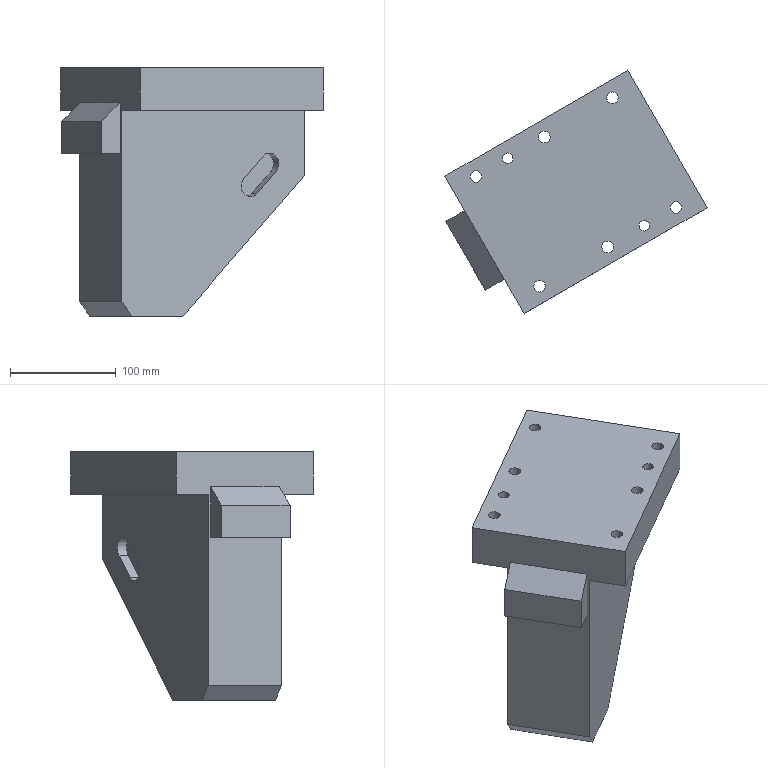Part | NX | features solid 2 | 1 solid | 47 faces | box 248.205 x 229.904 x 235 mm | volume 3610096 mm3 | plane 29 | cylinder 18 | commonest cylinder face diameters 11 x6 17 x6 20 x4 10 x2
STEP:
#1=CARTESIAN_POINT('',(-1183.369,-2.122,138.943));
#2=VERTEX_POINT('',#1);
#3=CARTESIAN_POINT('',(-1165.421,8.24,138.943));
#4=VERTEX_POINT('',#3);
#5=CARTESIAN_POINT('',(-1169.752,5.74,138.943));
#6=DIRECTION('',(-0.866,-0.5,0.));
#7=VECTOR('',#6,1000.);
#8=LINE('',#5,#7);
#9=EDGE_CURVE('',#2,#4,#8,.F.);
#10=ORIENTED_EDGE('',*,*,#9,.T.);
#11=CARTESIAN_POINT('',(-1127.921,-56.712,138.943));
#12=VERTEX_POINT('',#11);
#13=CARTESIAN_POINT('',(-1088.171,-125.561,138.943));
#14=DIRECTION('',(-0.5,0.866,0.));
#15=VECTOR('',#14,1000.);
#16=LINE('',#13,#15);
#17=EDGE_CURVE('',#12,#4,#16,.T.);
#18=ORIENTED_EDGE('',*,*,#17,.F.);
#19=CARTESIAN_POINT('',(-1145.869,-67.074,138.943));
#20=VERTEX_POINT('',#19);
#21=CARTESIAN_POINT('',(-1132.252,-59.212,138.943));
#22=DIRECTION('',(0.866,0.5,0.));
#23=VECTOR('',#22,1000.);
#24=LINE('',#21,#23);
#25=EDGE_CURVE('',#20,#12,#24,.T.);
#26=ORIENTED_EDGE('',*,*,#25,.F.);
#27=CARTESIAN_POINT('',(-1145.869,-67.074,138.943));
#28=DIRECTION('',(-0.5,0.866,0.));
#29=VECTOR('',#28,1000.);
#30=LINE('',#27,#29);
#31=EDGE_CURVE('',#20,#2,#30,.T.);
#32=ORIENTED_EDGE('',*,*,#31,.T.);
#33=EDGE_LOOP('',(#10,#18,#26,#32));
#34=FACE_BOUND('',#33,.T.);
#35=CARTESIAN_POINT('',(-1088.171,-125.561,138.943));
#36=DIRECTION('',(0.,0.,1.));
#37=DIRECTION('',(0.5,-0.866,0.));
#38=AXIS2_PLACEMENT_3D('',#35,#36,#37);
#39=PLANE('',#38);
#40=ADVANCED_FACE('',(#34),#39,.F.);
#41=CARTESIAN_POINT('',(-1145.869,-67.074,169.58));
#42=VERTEX_POINT('',#41);
#43=CARTESIAN_POINT('',(-1127.921,-56.712,186.97));
#44=VERTEX_POINT('',#43);
#45=CARTESIAN_POINT('',(-1129.327,-57.524,185.608));
#46=DIRECTION('',(0.6634,0.383,0.6428));
#47=VECTOR('',#46,1000.);
#48=LINE('',#45,#47);
#49=EDGE_CURVE('',#42,#44,#48,.T.);
#50=ORIENTED_EDGE('',*,*,#49,.T.);
#51=CARTESIAN_POINT('',(-1165.421,8.24,186.97));
#52=VERTEX_POINT('',#51);
#53=CARTESIAN_POINT('',(-1126.671,-58.877,186.97));
#54=DIRECTION('',(0.5,-0.866,0.));
#55=VECTOR('',#54,1000.);
#56=LINE('',#53,#55);
#57=EDGE_CURVE('',#52,#44,#56,.T.);
#58=ORIENTED_EDGE('',*,*,#57,.F.);
#59=CARTESIAN_POINT('',(-1183.369,-2.122,169.58));
#60=VERTEX_POINT('',#59);
#61=CARTESIAN_POINT('',(-1166.827,7.428,185.608));
#62=DIRECTION('',(-0.6634,-0.383,-0.6428));
#63=VECTOR('',#62,1000.);
#64=LINE('',#61,#63);
#65=EDGE_CURVE('',#60,#52,#64,.F.);
#66=ORIENTED_EDGE('',*,*,#65,.F.);
#67=CARTESIAN_POINT('',(-1145.869,-67.074,169.58));
#68=DIRECTION('',(0.5,-0.866,0.));
#69=VECTOR('',#68,1000.);
#70=LINE('',#67,#69);
#71=EDGE_CURVE('',#42,#60,#70,.F.);
#72=ORIENTED_EDGE('',*,*,#71,.F.);
#73=EDGE_LOOP('',(#50,#58,#66,#72));
#74=FACE_BOUND('',#73,.T.);
#75=CARTESIAN_POINT('',(-1128.077,-59.689,185.608));
#76=DIRECTION('',(0.5567,0.3214,-0.766));
#77=DIRECTION('',(-0.6313,-0.4358,-0.6416));
#78=AXIS2_PLACEMENT_3D('',#75,#76,#77);
#79=PLANE('',#78);
#80=ADVANCED_FACE('',(#74),#79,.F.);
#81=CARTESIAN_POINT('',(-998.759,14.973,101.136));
#82=VERTEX_POINT('',#81);
#83=CARTESIAN_POINT('',(-1011.006,7.902,115.279));
#84=VERTEX_POINT('',#83);
#85=CARTESIAN_POINT('',(-1004.882,11.438,108.208));
#86=DIRECTION('',(0.5,-0.866,0.));
#87=DIRECTION('',(0.866,0.5,0.));
#88=AXIS2_PLACEMENT_3D('',#85,#86,#87);
#89=CIRCLE('',#88,10.);
#90=EDGE_CURVE('',#82,#84,#89,.F.);
#91=ORIENTED_EDGE('',*,*,#90,.T.);
#92=CARTESIAN_POINT('',(-992.635,18.509,136.492));
#93=VERTEX_POINT('',#92);
#94=CARTESIAN_POINT('',(-1017.13,4.367,108.208));
#95=DIRECTION('',(0.6124,0.3536,0.7071));
#96=VECTOR('',#95,1000.);
#97=LINE('',#94,#96);
#98=EDGE_CURVE('',#93,#84,#97,.F.);
#99=ORIENTED_EDGE('',*,*,#98,.F.);
#100=CARTESIAN_POINT('',(-980.387,25.58,122.35));
#101=VERTEX_POINT('',#100);
#102=CARTESIAN_POINT('',(-986.511,22.044,129.421));
#103=DIRECTION('',(0.5,-0.866,0.));
#104=DIRECTION('',(0.866,0.5,0.));
#105=AXIS2_PLACEMENT_3D('',#102,#103,#104);
#106=CIRCLE('',#105,10.);
#107=EDGE_CURVE('',#93,#101,#106,.F.);
#108=ORIENTED_EDGE('',*,*,#107,.T.);
#109=CARTESIAN_POINT('',(-924.354,57.931,187.052));
#110=DIRECTION('',(-0.6124,-0.3536,-0.7071));
#111=VECTOR('',#110,1000.);
#112=LINE('',#109,#111);
#113=EDGE_CURVE('',#82,#101,#112,.F.);
#114=ORIENTED_EDGE('',*,*,#113,.F.);
#115=EDGE_LOOP('',(#91,#99,#108,#114));
#116=FACE_BOUND('',#115,.T.);
#117=CARTESIAN_POINT('',(-1126.671,-58.877,-1.401));
#118=VERTEX_POINT('',#117);
#119=CARTESIAN_POINT('',(-1116.79,-53.172,-15.));
#120=VERTEX_POINT('',#119);
#121=CARTESIAN_POINT('',(-1116.129,-52.791,-15.909));
#122=DIRECTION('',(-0.5567,-0.3214,0.766));
#123=VECTOR('',#122,1000.);
#124=LINE('',#121,#123);
#125=EDGE_CURVE('',#118,#120,#124,.F.);
#126=ORIENTED_EDGE('',*,*,#125,.T.);
#127=CARTESIAN_POINT('',(-1068.717,-25.417,-15.));
#128=VERTEX_POINT('',#127);
#129=CARTESIAN_POINT('',(-746.06,160.869,-15.));
#130=DIRECTION('',(-0.866,-0.5,0.));
#131=VECTOR('',#130,1000.);
#132=LINE('',#129,#131);
#133=EDGE_CURVE('',#120,#128,#132,.F.);
#134=ORIENTED_EDGE('',*,*,#133,.T.);
#135=CARTESIAN_POINT('',(-953.466,41.123,118.08));
#136=VERTEX_POINT('',#135);
#137=CARTESIAN_POINT('',(-1050.063,-14.647,6.54));
#138=DIRECTION('',(-0.6124,-0.3536,-0.7071));
#139=VECTOR('',#138,1000.);
#140=LINE('',#137,#139);
#141=EDGE_CURVE('',#128,#136,#140,.F.);
#142=ORIENTED_EDGE('',*,*,#141,.T.);
#143=CARTESIAN_POINT('',(-953.466,41.123,180.));
#144=VERTEX_POINT('',#143);
#145=CARTESIAN_POINT('',(-953.466,41.123,-270.576));
#146=DIRECTION('',(0.,0.,-1.));
#147=VECTOR('',#146,1000.);
#148=LINE('',#145,#147);
#149=EDGE_CURVE('',#136,#144,#148,.F.);
#150=ORIENTED_EDGE('',*,*,#149,.T.);
#151=CARTESIAN_POINT('',(-1126.671,-58.877,180.));
#152=VERTEX_POINT('',#151);
#153=CARTESIAN_POINT('',(-746.06,160.869,180.));
#154=DIRECTION('',(0.866,0.5,0.));
#155=VECTOR('',#154,1000.);
#156=LINE('',#153,#155);
#157=EDGE_CURVE('',#144,#152,#156,.F.);
#158=ORIENTED_EDGE('',*,*,#157,.T.);
#159=CARTESIAN_POINT('',(-1126.671,-58.877,-5.827));
#160=DIRECTION('',(0.,0.,-1.));
#161=VECTOR('',#160,1000.);
#162=LINE('',#159,#161);
#163=EDGE_CURVE('',#118,#152,#162,.F.);
#164=ORIENTED_EDGE('',*,*,#163,.F.);
#165=EDGE_LOOP('',(#126,#134,#142,#150,#158,#164));
#166=FACE_BOUND('',#165,.T.);
#167=CARTESIAN_POINT('',(-746.06,160.869,-18.824));
#168=DIRECTION('',(0.5,-0.866,0.));
#169=DIRECTION('',(0.8627,0.4981,-0.08716));
#170=AXIS2_PLACEMENT_3D('',#167,#168,#169);
#171=PLANE('',#170);
#172=ADVANCED_FACE('',(#116,#166),#171,.T.);
#173=CARTESIAN_POINT('',(-1016.006,16.562,115.279));
#174=VERTEX_POINT('',#173);
#175=CARTESIAN_POINT('',(-1003.759,23.634,101.136));
#176=VERTEX_POINT('',#175);
#177=CARTESIAN_POINT('',(-1009.882,20.098,108.208));
#178=DIRECTION('',(0.5,-0.866,0.));
#179=DIRECTION('',(0.866,0.5,0.));
#180=AXIS2_PLACEMENT_3D('',#177,#178,#179);
#181=CIRCLE('',#180,10.);
#182=EDGE_CURVE('',#174,#176,#181,.T.);
#183=ORIENTED_EDGE('',*,*,#182,.T.);
#184=CARTESIAN_POINT('',(-985.387,34.24,122.35));
#185=VERTEX_POINT('',#184);
#186=CARTESIAN_POINT('',(-1052.748,-4.651,44.568));
#187=DIRECTION('',(-0.6124,-0.3536,-0.7071));
#188=VECTOR('',#187,1000.);
#189=LINE('',#186,#188);
#190=EDGE_CURVE('',#176,#185,#189,.F.);
#191=ORIENTED_EDGE('',*,*,#190,.T.);
#192=CARTESIAN_POINT('',(-997.635,27.169,136.492));
#193=VERTEX_POINT('',#192);
#194=CARTESIAN_POINT('',(-991.511,30.705,129.421));
#195=DIRECTION('',(0.5,-0.866,0.));
#196=DIRECTION('',(0.866,0.5,0.));
#197=AXIS2_PLACEMENT_3D('',#194,#195,#196);
#198=CIRCLE('',#197,10.);
#199=EDGE_CURVE('',#185,#193,#198,.T.);
#200=ORIENTED_EDGE('',*,*,#199,.T.);
#201=CARTESIAN_POINT('',(-1064.996,-11.722,58.71));
#202=DIRECTION('',(-0.6124,-0.3536,-0.7071));
#203=VECTOR('',#202,1000.);
#204=LINE('',#201,#203);
#205=EDGE_CURVE('',#174,#193,#204,.F.);
#206=ORIENTED_EDGE('',*,*,#205,.F.);
#207=EDGE_LOOP('',(#183,#191,#200,#206));
#208=FACE_BOUND('',#207,.T.);
#209=CARTESIAN_POINT('',(-1052.748,-4.651,44.568));
#210=DIRECTION('',(0.5,-0.866,0.));
#211=DIRECTION('',(0.6124,0.3536,0.7071));
#212=AXIS2_PLACEMENT_3D('',#209,#210,#211);
#213=PLANE('',#212);
#214=ADVANCED_FACE('',(#208),#213,.T.);
#215=CARTESIAN_POINT('',(-1046.006,68.524,115.279));
#216=VERTEX_POINT('',#215);
#217=CARTESIAN_POINT('',(-1033.759,75.595,101.136));
#218=VERTEX_POINT('',#217);
#219=CARTESIAN_POINT('',(-1039.882,72.059,108.208));
#220=DIRECTION('',(-0.5,0.866,0.));
#221=DIRECTION('',(-0.8627,-0.4981,0.08716));
#222=AXIS2_PLACEMENT_3D('',#219,#220,#221);
#223=CIRCLE('',#222,10.);
#224=EDGE_CURVE('',#216,#218,#223,.F.);
#225=ORIENTED_EDGE('',*,*,#224,.F.);
#226=CARTESIAN_POINT('',(-1027.635,79.131,136.492));
#227=VERTEX_POINT('',#226);
#228=CARTESIAN_POINT('',(-1052.13,64.988,108.208));
#229=DIRECTION('',(-0.6124,-0.3536,-0.7071));
#230=VECTOR('',#229,1000.);
#231=LINE('',#228,#230);
#232=EDGE_CURVE('',#216,#227,#231,.F.);
#233=ORIENTED_EDGE('',*,*,#232,.T.);
#234=CARTESIAN_POINT('',(-1015.387,86.202,122.35));
#235=VERTEX_POINT('',#234);
#236=CARTESIAN_POINT('',(-1021.511,82.666,129.421));
#237=DIRECTION('',(-0.5,0.866,0.));
#238=DIRECTION('',(-0.8627,-0.4981,0.08716));
#239=AXIS2_PLACEMENT_3D('',#236,#237,#238);
#240=CIRCLE('',#239,10.);
#241=EDGE_CURVE('',#235,#227,#240,.F.);
#242=ORIENTED_EDGE('',*,*,#241,.F.);
#243=CARTESIAN_POINT('',(-1039.882,72.059,94.065));
#244=DIRECTION('',(-0.6124,-0.3536,-0.7071));
#245=VECTOR('',#244,1000.);
#246=LINE('',#243,#245);
#247=EDGE_CURVE('',#218,#235,#246,.F.);
#248=ORIENTED_EDGE('',*,*,#247,.F.);
#249=EDGE_LOOP('',(#225,#233,#242,#248));
#250=FACE_BOUND('',#249,.T.);
#251=CARTESIAN_POINT('',(-1082.748,47.311,44.568));
#252=DIRECTION('',(-0.5,0.866,0.));
#253=DIRECTION('',(0.6124,0.3536,0.7071));
#254=AXIS2_PLACEMENT_3D('',#251,#252,#253);
#255=PLANE('',#254);
#256=ADVANCED_FACE('',(#250),#255,.T.);
#257=ORIENTED_EDGE('',*,*,#113,.T.);
#258=CARTESIAN_POINT('',(-935.387,-52.362,122.35));
#259=DIRECTION('',(-0.5,0.866,0.));
#260=VECTOR('',#259,1000.);
#261=LINE('',#258,#260);
#262=EDGE_CURVE('',#101,#185,#261,.T.);
#263=ORIENTED_EDGE('',*,*,#262,.T.);
#264=ORIENTED_EDGE('',*,*,#190,.F.);
#265=CARTESIAN_POINT('',(-953.759,-62.969,101.136));
#266=DIRECTION('',(-0.5,0.866,0.));
#267=VECTOR('',#266,1000.);
#268=LINE('',#265,#267);
#269=EDGE_CURVE('',#82,#176,#268,.T.);
#270=ORIENTED_EDGE('',*,*,#269,.F.);
#271=EDGE_LOOP('',(#257,#263,#264,#270));
#272=FACE_BOUND('',#271,.T.);
#273=CARTESIAN_POINT('',(-959.882,-66.505,94.065));
#274=DIRECTION('',(-0.6124,-0.3536,0.7071));
#275=DIRECTION('',(-0.4824,-0.5415,-0.6885));
#276=AXIS2_PLACEMENT_3D('',#273,#274,#275);
#277=PLANE('',#276);
#278=ADVANCED_FACE('',(#272),#277,.T.);
#279=ORIENTED_EDGE('',*,*,#107,.F.);
#280=CARTESIAN_POINT('',(-947.635,-59.434,136.492));
#281=DIRECTION('',(-0.5,0.866,0.));
#282=VECTOR('',#281,1000.);
#283=LINE('',#280,#282);
#284=EDGE_CURVE('',#93,#193,#283,.T.);
#285=ORIENTED_EDGE('',*,*,#284,.T.);
#286=ORIENTED_EDGE('',*,*,#199,.F.);
#287=ORIENTED_EDGE('',*,*,#262,.F.);
#288=EDGE_LOOP('',(#279,#285,#286,#287));
#289=FACE_BOUND('',#288,.T.);
#290=CARTESIAN_POINT('',(-941.511,-55.898,129.421));
#291=DIRECTION('',(-0.5,0.866,0.));
#292=DIRECTION('',(-0.8627,-0.4981,0.08716));
#293=AXIS2_PLACEMENT_3D('',#290,#291,#292);
#294=CYLINDRICAL_SURFACE('',#293,10.);
#295=ADVANCED_FACE('',(#289),#294,.F.);
#296=ORIENTED_EDGE('',*,*,#284,.F.);
#297=ORIENTED_EDGE('',*,*,#98,.T.);
#298=CARTESIAN_POINT('',(-966.006,-70.04,115.279));
#299=DIRECTION('',(-0.5,0.866,0.));
#300=VECTOR('',#299,1000.);
#301=LINE('',#298,#300);
#302=EDGE_CURVE('',#84,#174,#301,.T.);
#303=ORIENTED_EDGE('',*,*,#302,.T.);
#304=ORIENTED_EDGE('',*,*,#205,.T.);
#305=EDGE_LOOP('',(#296,#297,#303,#304));
#306=FACE_BOUND('',#305,.T.);
#307=CARTESIAN_POINT('',(-972.13,-73.576,108.208));
#308=DIRECTION('',(-0.6124,-0.3536,0.7071));
#309=DIRECTION('',(-0.4824,-0.5415,-0.6885));
#310=AXIS2_PLACEMENT_3D('',#307,#308,#309);
#311=PLANE('',#310);
#312=ADVANCED_FACE('',(#306),#311,.F.);
#313=ORIENTED_EDGE('',*,*,#302,.F.);
#314=ORIENTED_EDGE('',*,*,#90,.F.);
#315=ORIENTED_EDGE('',*,*,#269,.T.);
#316=ORIENTED_EDGE('',*,*,#182,.F.);
#317=EDGE_LOOP('',(#313,#314,#315,#316));
#318=FACE_BOUND('',#317,.T.);
#319=CARTESIAN_POINT('',(-959.882,-66.505,108.208));
#320=DIRECTION('',(-0.5,0.866,0.));
#321=DIRECTION('',(-0.8627,-0.4981,0.08716));
#322=AXIS2_PLACEMENT_3D('',#319,#320,#321);
#323=CYLINDRICAL_SURFACE('',#322,10.);
#324=ADVANCED_FACE('',(#318),#323,.F.);
#325=ORIENTED_EDGE('',*,*,#241,.T.);
#326=CARTESIAN_POINT('',(-1032.635,87.791,136.492));
#327=VERTEX_POINT('',#326);
#328=CARTESIAN_POINT('',(-1032.635,87.791,136.492));
#329=DIRECTION('',(0.5,-0.866,0.));
#330=VECTOR('',#329,1000.);
#331=LINE('',#328,#330);
#332=EDGE_CURVE('',#227,#327,#331,.F.);
#333=ORIENTED_EDGE('',*,*,#332,.T.);
#334=CARTESIAN_POINT('',(-1020.387,94.862,122.35));
#335=VERTEX_POINT('',#334);
#336=CARTESIAN_POINT('',(-1026.511,91.326,129.421));
#337=DIRECTION('',(-0.5,0.866,0.));
#338=DIRECTION('',(-0.8627,-0.4981,0.08716));
#339=AXIS2_PLACEMENT_3D('',#336,#337,#338);
#340=CIRCLE('',#339,10.);
#341=EDGE_CURVE('',#327,#335,#340,.T.);
#342=ORIENTED_EDGE('',*,*,#341,.T.);
#343=CARTESIAN_POINT('',(-1017.887,90.532,122.35));
#344=DIRECTION('',(0.5,-0.866,0.));
#345=VECTOR('',#344,1000.);
#346=LINE('',#343,#345);
#347=EDGE_CURVE('',#335,#235,#346,.T.);
#348=ORIENTED_EDGE('',*,*,#347,.T.);
#349=EDGE_LOOP('',(#325,#333,#342,#348));
#350=FACE_BOUND('',#349,.T.);
#351=CARTESIAN_POINT('',(-1024.011,86.996,129.421));
#352=DIRECTION('',(-0.5,0.866,0.));
#353=DIRECTION('',(0.8627,0.4981,-0.08716));
#354=AXIS2_PLACEMENT_3D('',#351,#352,#353);
#355=CYLINDRICAL_SURFACE('',#354,10.);
#356=ADVANCED_FACE('',(#350),#355,.F.);
#357=ORIENTED_EDGE('',*,*,#247,.T.);
#358=ORIENTED_EDGE('',*,*,#347,.F.);
#359=CARTESIAN_POINT('',(-1038.759,84.255,101.136));
#360=VERTEX_POINT('',#359);
#361=CARTESIAN_POINT('',(-1044.882,80.72,94.065));
#362=DIRECTION('',(0.6124,0.3536,0.7071));
#363=VECTOR('',#362,1000.);
#364=LINE('',#361,#363);
#365=EDGE_CURVE('',#360,#335,#364,.T.);
#366=ORIENTED_EDGE('',*,*,#365,.F.);
#367=CARTESIAN_POINT('',(-1036.259,79.925,101.136));
#368=DIRECTION('',(-0.5,0.866,0.));
#369=VECTOR('',#368,1000.);
#370=LINE('',#367,#369);
#371=EDGE_CURVE('',#218,#360,#370,.T.);
#372=ORIENTED_EDGE('',*,*,#371,.F.);
#373=EDGE_LOOP('',(#357,#358,#366,#372));
#374=FACE_BOUND('',#373,.T.);
#375=CARTESIAN_POINT('',(-1042.382,76.39,94.065));
#376=DIRECTION('',(-0.6124,-0.3536,0.7071));
#377=DIRECTION('',(0.6124,0.3536,0.7071));
#378=AXIS2_PLACEMENT_3D('',#375,#376,#377);
#379=PLANE('',#378);
#380=ADVANCED_FACE('',(#374),#379,.T.);
#381=CARTESIAN_POINT('',(-1051.006,77.184,115.279));
#382=VERTEX_POINT('',#381);
#383=CARTESIAN_POINT('',(-1044.882,80.72,108.208));
#384=DIRECTION('',(-0.5,0.866,0.));
#385=DIRECTION('',(-0.8627,-0.4981,0.08716));
#386=AXIS2_PLACEMENT_3D('',#383,#384,#385);
#387=CIRCLE('',#386,10.);
#388=EDGE_CURVE('',#360,#382,#387,.T.);
#389=ORIENTED_EDGE('',*,*,#388,.T.);
#390=CARTESIAN_POINT('',(-1041.006,59.864,115.279));
#391=DIRECTION('',(-0.5,0.866,0.));
#392=VECTOR('',#391,1000.);
#393=LINE('',#390,#392);
#394=EDGE_CURVE('',#382,#216,#393,.F.);
#395=ORIENTED_EDGE('',*,*,#394,.T.);
#396=ORIENTED_EDGE('',*,*,#224,.T.);
#397=ORIENTED_EDGE('',*,*,#371,.T.);
#398=EDGE_LOOP('',(#389,#395,#396,#397));
#399=FACE_BOUND('',#398,.T.);
#400=CARTESIAN_POINT('',(-1042.382,76.39,108.208));
#401=DIRECTION('',(0.5,-0.866,0.));
#402=DIRECTION('',(-0.8627,-0.4981,0.08716));
#403=AXIS2_PLACEMENT_3D('',#400,#401,#402);
#404=CYLINDRICAL_SURFACE('',#403,10.);
#405=ADVANCED_FACE('',(#399),#404,.F.);
#406=CARTESIAN_POINT('',(-1088.495,55.54,71.99));
#407=DIRECTION('',(-0.6124,-0.3536,-0.7071));
#408=VECTOR('',#407,1000.);
#409=LINE('',#406,#408);
#410=EDGE_CURVE('',#327,#382,#409,.T.);
#411=ORIENTED_EDGE('',*,*,#410,.F.);
#412=ORIENTED_EDGE('',*,*,#332,.F.);
#413=ORIENTED_EDGE('',*,*,#232,.F.);
#414=ORIENTED_EDGE('',*,*,#394,.F.);
#415=EDGE_LOOP('',(#411,#412,#413,#414));
#416=FACE_BOUND('',#415,.T.);
#417=CARTESIAN_POINT('',(-1054.63,69.319,108.208));
#418=DIRECTION('',(-0.6124,-0.3536,0.7071));
#419=DIRECTION('',(0.6124,0.3536,0.7071));
#420=AXIS2_PLACEMENT_3D('',#417,#418,#419);
#421=PLANE('',#420);
#422=ADVANCED_FACE('',(#416),#421,.F.);
#423=ORIENTED_EDGE('',*,*,#125,.F.);
#424=CARTESIAN_POINT('',(-1166.671,10.405,-1.401));
#425=VERTEX_POINT('',#424);
#426=CARTESIAN_POINT('',(-1082.171,-135.954,-1.401));
#427=DIRECTION('',(0.5,-0.866,0.));
#428=VECTOR('',#427,1000.);
#429=LINE('',#426,#428);
#430=EDGE_CURVE('',#425,#118,#429,.T.);
#431=ORIENTED_EDGE('',*,*,#430,.F.);
#432=CARTESIAN_POINT('',(-1156.79,16.11,-15.));
#433=VERTEX_POINT('',#432);
#434=CARTESIAN_POINT('',(-1114.438,40.562,-73.281));
#435=DIRECTION('',(-0.5567,-0.3214,0.766));
#436=VECTOR('',#435,1000.);
#437=LINE('',#434,#436);
#438=EDGE_CURVE('',#433,#425,#437,.T.);
#439=ORIENTED_EDGE('',*,*,#438,.F.);
#440=CARTESIAN_POINT('',(-1072.29,-130.248,-15.));
#441=DIRECTION('',(-0.5,0.866,0.));
#442=VECTOR('',#441,1000.);
#443=LINE('',#440,#442);
#444=EDGE_CURVE('',#120,#433,#443,.T.);
#445=ORIENTED_EDGE('',*,*,#444,.F.);
#446=EDGE_LOOP('',(#423,#431,#439,#445));
#447=FACE_BOUND('',#446,.T.);
#448=CARTESIAN_POINT('',(-1071.629,-129.867,-15.909));
#449=DIRECTION('',(-0.6634,-0.383,-0.6428));
#450=DIRECTION('',(-0.5247,-0.3743,0.7646));
#451=AXIS2_PLACEMENT_3D('',#448,#449,#450);
#452=PLANE('',#451);
#453=ADVANCED_FACE('',(#447),#452,.T.);
#454=CARTESIAN_POINT('',(-1108.717,43.865,-15.));
#455=VERTEX_POINT('',#454);
#456=CARTESIAN_POINT('',(-1103.275,34.439,-15.));
#457=DIRECTION('',(0.5,-0.866,0.));
#458=VECTOR('',#457,1000.);
#459=LINE('',#456,#458);
#460=EDGE_CURVE('',#455,#128,#459,.T.);
#461=ORIENTED_EDGE('',*,*,#460,.F.);
#462=CARTESIAN_POINT('',(-993.466,110.405,118.08));
#463=VERTEX_POINT('',#462);
#464=CARTESIAN_POINT('',(-1090.063,54.635,6.54));
#465=DIRECTION('',(-0.6124,-0.3536,-0.7071));
#466=VECTOR('',#465,1000.);
#467=LINE('',#464,#466);
#468=EDGE_CURVE('',#463,#455,#467,.T.);
#469=ORIENTED_EDGE('',*,*,#468,.F.);
#470=CARTESIAN_POINT('',(-880.966,-84.451,118.08));
#471=DIRECTION('',(-0.5,0.866,0.));
#472=VECTOR('',#471,1000.);
#473=LINE('',#470,#472);
#474=EDGE_CURVE('',#136,#463,#473,.T.);
#475=ORIENTED_EDGE('',*,*,#474,.F.);
#476=ORIENTED_EDGE('',*,*,#141,.F.);
#477=EDGE_LOOP('',(#461,#469,#475,#476));
#478=FACE_BOUND('',#477,.T.);
#479=CARTESIAN_POINT('',(-1084.621,45.209,6.54));
#480=DIRECTION('',(0.6124,0.3536,-0.7071));
#481=DIRECTION('',(0.5,-0.866,0.));
#482=AXIS2_PLACEMENT_3D('',#479,#480,#481);
#483=PLANE('',#482);
#484=ADVANCED_FACE('',(#478),#483,.T.);
#485=CARTESIAN_POINT('',(-993.466,110.405,180.));
#486=VERTEX_POINT('',#485);
#487=CARTESIAN_POINT('',(-993.466,110.405,-270.576));
#488=DIRECTION('',(0.,0.,1.));
#489=VECTOR('',#488,1000.);
#490=LINE('',#487,#489);
#491=EDGE_CURVE('',#463,#486,#490,.T.);
#492=ORIENTED_EDGE('',*,*,#491,.T.);
#493=CARTESIAN_POINT('',(-1010.966,140.716,180.));
#494=VERTEX_POINT('',#493);
#495=CARTESIAN_POINT('',(-880.966,-84.451,180.));
#496=DIRECTION('',(-0.5,0.866,0.));
#497=VECTOR('',#496,1000.);
#498=LINE('',#495,#497);
#499=EDGE_CURVE('',#486,#494,#498,.T.);
#500=ORIENTED_EDGE('',*,*,#499,.T.);
#501=CARTESIAN_POINT('',(-1010.966,140.716,220.));
#502=VERTEX_POINT('',#501);
#503=CARTESIAN_POINT('',(-1010.966,140.716,-270.576));
#504=DIRECTION('',(0.,0.,-1.));
#505=VECTOR('',#504,1000.);
#506=LINE('',#503,#505);
#507=EDGE_CURVE('',#502,#494,#506,.T.);
#508=ORIENTED_EDGE('',*,*,#507,.F.);
#509=CARTESIAN_POINT('',(-935.966,10.812,220.));
#510=VERTEX_POINT('',#509);
#511=CARTESIAN_POINT('',(-880.966,-84.451,220.));
#512=DIRECTION('',(-0.5,0.866,0.));
#513=VECTOR('',#512,1000.);
#514=LINE('',#511,#513);
#515=EDGE_CURVE('',#510,#502,#514,.T.);
#516=ORIENTED_EDGE('',*,*,#515,.F.);
#517=CARTESIAN_POINT('',(-935.966,10.812,180.));
#518=VERTEX_POINT('',#517);
#519=CARTESIAN_POINT('',(-935.966,10.812,-270.576));
#520=DIRECTION('',(0.,0.,1.));
#521=VECTOR('',#520,1000.);
#522=LINE('',#519,#521);
#523=EDGE_CURVE('',#518,#510,#522,.T.);
#524=ORIENTED_EDGE('',*,*,#523,.F.);
#525=CARTESIAN_POINT('',(-880.966,-84.451,180.));
#526=DIRECTION('',(-0.5,0.866,0.));
#527=VECTOR('',#526,1000.);
#528=LINE('',#525,#527);
#529=EDGE_CURVE('',#518,#144,#528,.T.);
#530=ORIENTED_EDGE('',*,*,#529,.T.);
#531=ORIENTED_EDGE('',*,*,#149,.F.);
#532=ORIENTED_EDGE('',*,*,#474,.T.);
#533=EDGE_LOOP('',(#492,#500,#508,#516,#524,#530,#531,#532));
#534=FACE_BOUND('',#533,.T.);
#535=CARTESIAN_POINT('',(-880.966,-84.451,-270.576));
#536=DIRECTION('',(0.866,0.5,0.));
#537=DIRECTION('',(0.5,-0.866,0.));
#538=AXIS2_PLACEMENT_3D('',#535,#536,#537);
#539=PLANE('',#538);
#540=ADVANCED_FACE('',(#534),#539,.T.);
#541=ORIENTED_EDGE('',*,*,#468,.T.);
#542=CARTESIAN_POINT('',(-1078.54,61.288,-15.));
#543=DIRECTION('',(0.866,0.5,0.));
#544=VECTOR('',#543,1000.);
#545=LINE('',#542,#544);
#546=EDGE_CURVE('',#433,#455,#545,.T.);
#547=ORIENTED_EDGE('',*,*,#546,.F.);
#548=ORIENTED_EDGE('',*,*,#438,.T.);
#549=CARTESIAN_POINT('',(-1166.671,10.405,180.));
#550=VERTEX_POINT('',#549);
#551=CARTESIAN_POINT('',(-1166.671,10.405,-5.827));
#552=DIRECTION('',(0.,0.,1.));
#553=VECTOR('',#552,1000.);
#554=LINE('',#551,#553);
#555=EDGE_CURVE('',#425,#550,#554,.T.);
#556=ORIENTED_EDGE('',*,*,#555,.T.);
#557=CARTESIAN_POINT('',(-1078.54,61.288,180.));
#558=DIRECTION('',(-0.866,-0.5,0.));
#559=VECTOR('',#558,1000.);
#560=LINE('',#557,#559);
#561=EDGE_CURVE('',#486,#550,#560,.T.);
#562=ORIENTED_EDGE('',*,*,#561,.F.);
#563=ORIENTED_EDGE('',*,*,#491,.F.);
#564=EDGE_LOOP('',(#541,#547,#548,#556,#562,#563));
#565=FACE_BOUND('',#564,.T.);
#566=ORIENTED_EDGE('',*,*,#410,.T.);
#567=ORIENTED_EDGE('',*,*,#388,.F.);
#568=ORIENTED_EDGE('',*,*,#365,.T.);
#569=ORIENTED_EDGE('',*,*,#341,.F.);
#570=EDGE_LOOP('',(#566,#567,#568,#569));
#571=FACE_BOUND('',#570,.T.);
#572=CARTESIAN_POINT('',(-1078.54,61.288,-38.5));
#573=DIRECTION('',(-0.5,0.866,0.));
#574=DIRECTION('',(0.07548,0.04358,0.9962));
#575=AXIS2_PLACEMENT_3D('',#572,#573,#574);
#576=PLANE('',#575);
#577=ADVANCED_FACE('',(#565,#571),#576,.T.);
#578=CARTESIAN_POINT('',(-1165.421,8.24,204.173));
#579=DIRECTION('',(0.,0.,1.));
#580=VECTOR('',#579,1000.);
#581=LINE('',#578,#580);
#582=EDGE_CURVE('',#52,#4,#581,.F.);
#583=ORIENTED_EDGE('',*,*,#582,.F.);
#584=ORIENTED_EDGE('',*,*,#57,.T.);
#585=CARTESIAN_POINT('',(-1127.921,-56.712,154.173));
#586=DIRECTION('',(0.,0.,1.));
#587=VECTOR('',#586,1000.);
#588=LINE('',#585,#587);
#589=EDGE_CURVE('',#44,#12,#588,.F.);
#590=ORIENTED_EDGE('',*,*,#589,.T.);
#591=ORIENTED_EDGE('',*,*,#17,.T.);
#592=EDGE_LOOP('',(#583,#584,#590,#591));
#593=FACE_BOUND('',#592,.T.);
#594=ORIENTED_EDGE('',*,*,#555,.F.);
#595=ORIENTED_EDGE('',*,*,#430,.T.);
#596=ORIENTED_EDGE('',*,*,#163,.T.);
#597=CARTESIAN_POINT('',(-1109.171,-89.188,180.));
#598=VERTEX_POINT('',#597);
#599=CARTESIAN_POINT('',(-1082.171,-135.954,180.));
#600=DIRECTION('',(0.5,-0.866,0.));
#601=VECTOR('',#600,1000.);
#602=LINE('',#599,#601);
#603=EDGE_CURVE('',#152,#598,#602,.T.);
#604=ORIENTED_EDGE('',*,*,#603,.T.);
#605=CARTESIAN_POINT('',(-1109.171,-89.188,220.));
#606=VERTEX_POINT('',#605);
#607=CARTESIAN_POINT('',(-1109.171,-89.188,-20.576));
#608=DIRECTION('',(0.,0.,-1.));
#609=VECTOR('',#608,1000.);
#610=LINE('',#607,#609);
#611=EDGE_CURVE('',#598,#606,#610,.F.);
#612=ORIENTED_EDGE('',*,*,#611,.T.);
#613=CARTESIAN_POINT('',(-1184.171,40.716,220.));
#614=VERTEX_POINT('',#613);
#615=CARTESIAN_POINT('',(-1086.921,-127.726,220.));
#616=DIRECTION('',(-0.5,0.866,0.));
#617=VECTOR('',#616,1000.);
#618=LINE('',#615,#617);
#619=EDGE_CURVE('',#606,#614,#618,.T.);
#620=ORIENTED_EDGE('',*,*,#619,.T.);
#621=CARTESIAN_POINT('',(-1184.171,40.716,180.));
#622=VERTEX_POINT('',#621);
#623=CARTESIAN_POINT('',(-1184.171,40.716,144.424));
#624=DIRECTION('',(0.,0.,1.));
#625=VECTOR('',#624,1000.);
#626=LINE('',#623,#625);
#627=EDGE_CURVE('',#614,#622,#626,.F.);
#628=ORIENTED_EDGE('',*,*,#627,.T.);
#629=CARTESIAN_POINT('',(-1082.171,-135.954,180.));
#630=DIRECTION('',(0.5,-0.866,0.));
#631=VECTOR('',#630,1000.);
#632=LINE('',#629,#631);
#633=EDGE_CURVE('',#622,#550,#632,.T.);
#634=ORIENTED_EDGE('',*,*,#633,.T.);
#635=EDGE_LOOP('',(#594,#595,#596,#604,#612,#620,#628,#634));
#636=FACE_BOUND('',#635,.T.);
#637=CARTESIAN_POINT('',(-1086.921,-127.726,-5.827));
#638=DIRECTION('',(0.866,0.5,0.));
#639=DIRECTION('',(0.,0.,-1.));
#640=AXIS2_PLACEMENT_3D('',#637,#638,#639);
#641=PLANE('',#640);
#642=ADVANCED_FACE('',(#593,#636),#641,.F.);
#643=CARTESIAN_POINT('',(-995.428,-1.198,180.));
#644=VERTEX_POINT('',#643);
#645=CARTESIAN_POINT('',(-995.428,-6.198,180.));
#646=DIRECTION('',(0.,0.,-1.));
#647=DIRECTION('',(0.,1.,0.));
#648=AXIS2_PLACEMENT_3D('',#645,#646,#647);
#649=CIRCLE('',#648,5.);
#650=EDGE_CURVE('',#644,#644,#649,.F.);
#651=ORIENTED_EDGE('',*,*,#650,.T.);
#652=EDGE_LOOP('',(#651));
#653=FACE_BOUND('',#652,.T.);
#654=CARTESIAN_POINT('',(-965.55,19.552,180.));
#655=VERTEX_POINT('',#654);
#656=CARTESIAN_POINT('',(-965.55,11.052,180.));
#657=DIRECTION('',(0.,0.,-1.));
#658=DIRECTION('',(0.,1.,0.));
#659=AXIS2_PLACEMENT_3D('',#656,#657,#658);
#660=CIRCLE('',#659,8.5);
#661=EDGE_CURVE('',#655,#655,#660,.F.);
#662=ORIENTED_EDGE('',*,*,#661,.T.);
#663=EDGE_LOOP('',(#662));
#664=FACE_BOUND('',#663,.T.);
#665=CARTESIAN_POINT('',(-1094.588,-54.948,180.));
#666=VERTEX_POINT('',#665);
#667=CARTESIAN_POINT('',(-1094.588,-63.448,180.));
#668=DIRECTION('',(0.,0.,-1.));
#669=DIRECTION('',(0.,1.,0.));
#670=AXIS2_PLACEMENT_3D('',#667,#668,#669);
#671=CIRCLE('',#670,8.5);
#672=EDGE_CURVE('',#666,#666,#671,.F.);
#673=ORIENTED_EDGE('',*,*,#672,.T.);
#674=EDGE_LOOP('',(#673));
#675=FACE_BOUND('',#674,.T.);
#676=CARTESIAN_POINT('',(-1030.069,-17.698,180.));
#677=VERTEX_POINT('',#676);
#678=CARTESIAN_POINT('',(-1030.069,-26.198,180.));
#679=DIRECTION('',(0.,0.,-1.));
#680=DIRECTION('',(0.,1.,0.));
#681=AXIS2_PLACEMENT_3D('',#678,#679,#680);
#682=CIRCLE('',#681,8.5);
#683=EDGE_CURVE('',#677,#677,#682,.T.);
#684=ORIENTED_EDGE('',*,*,#683,.F.);
#685=EDGE_LOOP('',(#684));
#686=FACE_BOUND('',#685,.T.);
#687=ORIENTED_EDGE('',*,*,#157,.F.);
#688=ORIENTED_EDGE('',*,*,#529,.F.);
#689=CARTESIAN_POINT('',(-1212.229,-148.688,180.));
#690=DIRECTION('',(0.866,0.5,0.));
#691=VECTOR('',#690,1000.);
#692=LINE('',#689,#691);
#693=EDGE_CURVE('',#598,#518,#692,.T.);
#694=ORIENTED_EDGE('',*,*,#693,.F.);
#695=ORIENTED_EDGE('',*,*,#603,.F.);
#696=EDGE_LOOP('',(#687,#688,#694,#695));
#697=FACE_BOUND('',#696,.T.);
#698=CARTESIAN_POINT('',(-961.553,-66.314,180.));
#699=DIRECTION('',(0.,0.,-1.));
#700=DIRECTION('',(-0.866,-0.5,0.));
#701=AXIS2_PLACEMENT_3D('',#698,#699,#700);
#702=PLANE('',#701);
#703=ADVANCED_FACE('',(#653,#664,#675,#686,#697),#702,.T.);
#704=CARTESIAN_POINT('',(-1090.069,83.225,220.));
#705=VERTEX_POINT('',#704);
#706=CARTESIAN_POINT('',(-1090.069,77.725,220.));
#707=DIRECTION('',(0.,0.,-1.));
#708=DIRECTION('',(0.,1.,0.));
#709=AXIS2_PLACEMENT_3D('',#706,#707,#708);
#710=CIRCLE('',#709,5.5);
#711=EDGE_CURVE('',#705,#705,#710,.F.);
#712=ORIENTED_EDGE('',*,*,#711,.F.);
#713=EDGE_LOOP('',(#712));
#714=FACE_BOUND('',#713,.T.);
#715=CARTESIAN_POINT('',(-1094.588,-57.948,220.));
#716=VERTEX_POINT('',#715);
#717=CARTESIAN_POINT('',(-1094.588,-63.448,220.));
#718=DIRECTION('',(0.,0.,-1.));
#719=DIRECTION('',(0.,1.,0.));
#720=AXIS2_PLACEMENT_3D('',#717,#718,#719);
#721=CIRCLE('',#720,5.5);
#722=EDGE_CURVE('',#716,#716,#721,.T.);
#723=ORIENTED_EDGE('',*,*,#722,.T.);
#724=EDGE_LOOP('',(#723));
#725=FACE_BOUND('',#724,.T.);
#726=CARTESIAN_POINT('',(-965.55,16.552,220.));
#727=VERTEX_POINT('',#726);
#728=CARTESIAN_POINT('',(-965.55,11.052,220.));
#729=DIRECTION('',(0.,0.,-1.));
#730=DIRECTION('',(0.,1.,0.));
#731=AXIS2_PLACEMENT_3D('',#728,#729,#730);
#732=CIRCLE('',#731,5.5);
#733=EDGE_CURVE('',#727,#727,#732,.T.);
#734=ORIENTED_EDGE('',*,*,#733,.T.);
#735=EDGE_LOOP('',(#734));
#736=FACE_BOUND('',#735,.T.);
#737=CARTESIAN_POINT('',(-1154.588,45.975,220.));
#738=VERTEX_POINT('',#737);
#739=CARTESIAN_POINT('',(-1154.588,40.475,220.));
#740=DIRECTION('',(0.,0.,-1.));
#741=DIRECTION('',(0.,1.,0.));
#742=AXIS2_PLACEMENT_3D('',#739,#740,#741);
#743=CIRCLE('',#742,5.5);
#744=EDGE_CURVE('',#738,#738,#743,.T.);
#745=ORIENTED_EDGE('',*,*,#744,.T.);
#746=EDGE_LOOP('',(#745));
#747=FACE_BOUND('',#746,.T.);
#748=CARTESIAN_POINT('',(-1025.55,120.475,220.));
#749=VERTEX_POINT('',#748);
#750=CARTESIAN_POINT('',(-1025.55,114.975,220.));
#751=DIRECTION('',(0.,0.,-1.));
#752=DIRECTION('',(0.,1.,0.));
#753=AXIS2_PLACEMENT_3D('',#750,#751,#752);
#754=CIRCLE('',#753,5.5);
#755=EDGE_CURVE('',#749,#749,#754,.T.);
#756=ORIENTED_EDGE('',*,*,#755,.T.);
#757=EDGE_LOOP('',(#756));
#758=FACE_BOUND('',#757,.T.);
#759=CARTESIAN_POINT('',(-995.428,-1.198,220.));
#760=VERTEX_POINT('',#759);
#761=CARTESIAN_POINT('',(-995.428,-6.198,220.));
#762=DIRECTION('',(0.,0.,-1.));
#763=DIRECTION('',(0.,1.,0.));
#764=AXIS2_PLACEMENT_3D('',#761,#762,#763);
#765=CIRCLE('',#764,5.);
#766=EDGE_CURVE('',#760,#760,#765,.T.);
#767=ORIENTED_EDGE('',*,*,#766,.T.);
#768=EDGE_LOOP('',(#767));
#769=FACE_BOUND('',#768,.T.);
#770=CARTESIAN_POINT('',(-1124.71,62.725,220.));
#771=VERTEX_POINT('',#770);
#772=CARTESIAN_POINT('',(-1124.71,57.725,220.));
#773=DIRECTION('',(0.,0.,-1.));
#774=DIRECTION('',(0.,1.,0.));
#775=AXIS2_PLACEMENT_3D('',#772,#773,#774);
#776=CIRCLE('',#775,5.);
#777=EDGE_CURVE('',#771,#771,#776,.T.);
#778=ORIENTED_EDGE('',*,*,#777,.T.);
#779=EDGE_LOOP('',(#778));
#780=FACE_BOUND('',#779,.T.);
#781=ORIENTED_EDGE('',*,*,#619,.F.);
#782=CARTESIAN_POINT('',(-1212.229,-148.688,220.));
#783=DIRECTION('',(0.866,0.5,0.));
#784=VECTOR('',#783,1000.);
#785=LINE('',#782,#784);
#786=EDGE_CURVE('',#606,#510,#785,.T.);
#787=ORIENTED_EDGE('',*,*,#786,.T.);
#788=ORIENTED_EDGE('',*,*,#515,.T.);
#789=CARTESIAN_POINT('',(-1119.22,78.216,220.));
#790=DIRECTION('',(-0.866,-0.5,0.));
#791=VECTOR('',#790,1000.);
#792=LINE('',#789,#791);
#793=EDGE_CURVE('',#502,#614,#792,.T.);
#794=ORIENTED_EDGE('',*,*,#793,.T.);
#795=EDGE_LOOP('',(#781,#787,#788,#794));
#796=FACE_BOUND('',#795,.T.);
#797=CARTESIAN_POINT('',(-1030.069,-20.698,220.));
#798=VERTEX_POINT('',#797);
#799=CARTESIAN_POINT('',(-1030.069,-26.198,220.));
#800=DIRECTION('',(0.,0.,-1.));
#801=DIRECTION('',(0.,1.,0.));
#802=AXIS2_PLACEMENT_3D('',#799,#800,#801);
#803=CIRCLE('',#802,5.5);
#804=EDGE_CURVE('',#798,#798,#803,.F.);
#805=ORIENTED_EDGE('',*,*,#804,.F.);
#806=EDGE_LOOP('',(#805));
#807=FACE_BOUND('',#806,.T.);
#808=CARTESIAN_POINT('',(-1017.22,-98.454,220.));
#809=DIRECTION('',(0.,0.,-1.));
#810=DIRECTION('',(-0.5,0.866,0.));
#811=AXIS2_PLACEMENT_3D('',#808,#809,#810);
#812=PLANE('',#811);
#813=ADVANCED_FACE('',(#714,#725,#736,#747,#758,#769,#780,#796,#807),#812,.F.);
#814=ORIENTED_EDGE('',*,*,#499,.F.);
#815=ORIENTED_EDGE('',*,*,#561,.T.);
#816=ORIENTED_EDGE('',*,*,#633,.F.);
#817=CARTESIAN_POINT('',(-1063.553,110.355,180.));
#818=DIRECTION('',(-0.866,-0.5,0.));
#819=VECTOR('',#818,1000.);
#820=LINE('',#817,#819);
#821=EDGE_CURVE('',#494,#622,#820,.T.);
#822=ORIENTED_EDGE('',*,*,#821,.F.);
#823=EDGE_LOOP('',(#814,#815,#816,#822));
#824=FACE_BOUND('',#823,.T.);
#825=CARTESIAN_POINT('',(-1090.069,86.225,180.));
#826=VERTEX_POINT('',#825);
#827=CARTESIAN_POINT('',(-1090.069,77.725,180.));
#828=DIRECTION('',(0.,0.,-1.));
#829=DIRECTION('',(0.,1.,0.));
#830=AXIS2_PLACEMENT_3D('',#827,#828,#829);
#831=CIRCLE('',#830,8.5);
#832=EDGE_CURVE('',#826,#826,#831,.F.);
#833=ORIENTED_EDGE('',*,*,#832,.T.);
#834=EDGE_LOOP('',(#833));
#835=FACE_BOUND('',#834,.T.);
#836=CARTESIAN_POINT('',(-1124.71,62.725,180.));
#837=VERTEX_POINT('',#836);
#838=CARTESIAN_POINT('',(-1124.71,57.725,180.));
#839=DIRECTION('',(0.,0.,-1.));
#840=DIRECTION('',(0.,1.,0.));
#841=AXIS2_PLACEMENT_3D('',#838,#839,#840);
#842=CIRCLE('',#841,5.);
#843=EDGE_CURVE('',#837,#837,#842,.F.);
#844=ORIENTED_EDGE('',*,*,#843,.T.);
#845=EDGE_LOOP('',(#844));
#846=FACE_BOUND('',#845,.T.);
#847=CARTESIAN_POINT('',(-1025.55,123.475,180.));
#848=VERTEX_POINT('',#847);
#849=CARTESIAN_POINT('',(-1025.55,114.975,180.));
#850=DIRECTION('',(0.,0.,-1.));
#851=DIRECTION('',(0.,1.,0.));
#852=AXIS2_PLACEMENT_3D('',#849,#850,#851);
#853=CIRCLE('',#852,8.5);
#854=EDGE_CURVE('',#848,#848,#853,.F.);
#855=ORIENTED_EDGE('',*,*,#854,.T.);
#856=EDGE_LOOP('',(#855));
#857=FACE_BOUND('',#856,.T.);
#858=CARTESIAN_POINT('',(-1154.588,48.975,180.));
#859=VERTEX_POINT('',#858);
#860=CARTESIAN_POINT('',(-1154.588,40.475,180.));
#861=DIRECTION('',(0.,0.,-1.));
#862=DIRECTION('',(0.,1.,0.));
#863=AXIS2_PLACEMENT_3D('',#860,#861,#862);
#864=CIRCLE('',#863,8.5);
#865=EDGE_CURVE('',#859,#859,#864,.F.);
#866=ORIENTED_EDGE('',*,*,#865,.T.);
#867=EDGE_LOOP('',(#866));
#868=FACE_BOUND('',#867,.T.);
#869=CARTESIAN_POINT('',(-961.553,-66.314,180.));
#870=DIRECTION('',(0.,0.,-1.));
#871=DIRECTION('',(-0.866,-0.5,0.));
#872=AXIS2_PLACEMENT_3D('',#869,#870,#871);
#873=PLANE('',#872);
#874=ADVANCED_FACE('',(#824,#835,#846,#857,#868),#873,.T.);
#875=ORIENTED_EDGE('',*,*,#507,.T.);
#876=ORIENTED_EDGE('',*,*,#821,.T.);
#877=ORIENTED_EDGE('',*,*,#627,.F.);
#878=ORIENTED_EDGE('',*,*,#793,.F.);
#879=EDGE_LOOP('',(#875,#876,#877,#878));
#880=FACE_BOUND('',#879,.T.);
#881=CARTESIAN_POINT('',(-1063.553,110.355,144.424));
#882=DIRECTION('',(0.5,-0.866,0.));
#883=DIRECTION('',(0.,0.,-1.));
#884=AXIS2_PLACEMENT_3D('',#881,#882,#883);
#885=PLANE('',#884);
#886=ADVANCED_FACE('',(#880),#885,.F.);
#887=ORIENTED_EDGE('',*,*,#693,.T.);
#888=ORIENTED_EDGE('',*,*,#523,.T.);
#889=ORIENTED_EDGE('',*,*,#786,.F.);
#890=ORIENTED_EDGE('',*,*,#611,.F.);
#891=EDGE_LOOP('',(#887,#888,#889,#890));
#892=FACE_BOUND('',#891,.T.);
#893=CARTESIAN_POINT('',(-1212.229,-148.688,-270.576));
#894=DIRECTION('',(0.5,-0.866,0.));
#895=DIRECTION('',(-0.866,-0.5,0.));
#896=AXIS2_PLACEMENT_3D('',#893,#894,#895);
#897=PLANE('',#896);
#898=ADVANCED_FACE('',(#892),#897,.T.);
#899=CARTESIAN_POINT('',(-1094.588,-68.948,191.424));
#900=VERTEX_POINT('',#899);
#901=CARTESIAN_POINT('',(-1094.588,-63.448,191.424));
#902=DIRECTION('',(0.,0.,1.));
#903=DIRECTION('',(0.,-1.,0.));
#904=AXIS2_PLACEMENT_3D('',#901,#902,#903);
#905=CIRCLE('',#904,5.5);
#906=EDGE_CURVE('',#900,#900,#905,.T.);
#907=ORIENTED_EDGE('',*,*,#906,.F.);
#908=EDGE_LOOP('',(#907));
#909=FACE_BOUND('',#908,.T.);
#910=ORIENTED_EDGE('',*,*,#722,.F.);
#911=EDGE_LOOP('',(#910));
#912=FACE_BOUND('',#911,.T.);
#913=CARTESIAN_POINT('',(-1094.588,-63.448,144.424));
#914=DIRECTION('',(0.,0.,1.));
#915=DIRECTION('',(0.1736,-0.9848,0.));
#916=AXIS2_PLACEMENT_3D('',#913,#914,#915);
#917=CYLINDRICAL_SURFACE('',#916,5.5);
#918=ADVANCED_FACE('',(#909,#912),#917,.F.);
#919=ORIENTED_EDGE('',*,*,#906,.T.);
#920=EDGE_LOOP('',(#919));
#921=FACE_BOUND('',#920,.T.);
#922=CARTESIAN_POINT('',(-1094.588,-71.948,191.424));
#923=VERTEX_POINT('',#922);
#924=CARTESIAN_POINT('',(-1094.588,-63.448,191.424));
#925=DIRECTION('',(0.,0.,1.));
#926=DIRECTION('',(0.,-1.,0.));
#927=AXIS2_PLACEMENT_3D('',#924,#925,#926);
#928=CIRCLE('',#927,8.5);
#929=EDGE_CURVE('',#923,#923,#928,.T.);
#930=ORIENTED_EDGE('',*,*,#929,.F.);
#931=EDGE_LOOP('',(#930));
#932=FACE_BOUND('',#931,.T.);
#933=CARTESIAN_POINT('',(-1043.861,-132.31,191.424));
#934=DIRECTION('',(0.,0.,1.));
#935=DIRECTION('',(0.1736,-0.9848,0.));
#936=AXIS2_PLACEMENT_3D('',#933,#934,#935);
#937=PLANE('',#936);
#938=ADVANCED_FACE('',(#921,#932),#937,.F.);
#939=ORIENTED_EDGE('',*,*,#929,.T.);
#940=EDGE_LOOP('',(#939));
#941=FACE_BOUND('',#940,.T.);
#942=ORIENTED_EDGE('',*,*,#672,.F.);
#943=EDGE_LOOP('',(#942));
#944=FACE_BOUND('',#943,.T.);
#945=CARTESIAN_POINT('',(-1094.588,-63.448,94.424));
#946=DIRECTION('',(0.,0.,1.));
#947=DIRECTION('',(0.1736,-0.9848,0.));
#948=AXIS2_PLACEMENT_3D('',#945,#946,#947);
#949=CYLINDRICAL_SURFACE('',#948,8.5);
#950=ADVANCED_FACE('',(#941,#944),#949,.F.);
#951=CARTESIAN_POINT('',(-965.55,5.552,191.424));
#952=VERTEX_POINT('',#951);
#953=CARTESIAN_POINT('',(-965.55,11.052,191.424));
#954=DIRECTION('',(0.,0.,1.));
#955=DIRECTION('',(0.,-1.,0.));
#956=AXIS2_PLACEMENT_3D('',#953,#954,#955);
#957=CIRCLE('',#956,5.5);
#958=EDGE_CURVE('',#952,#952,#957,.T.);
#959=ORIENTED_EDGE('',*,*,#958,.F.);
#960=EDGE_LOOP('',(#959));
#961=FACE_BOUND('',#960,.T.);
#962=ORIENTED_EDGE('',*,*,#733,.F.);
#963=EDGE_LOOP('',(#962));
#964=FACE_BOUND('',#963,.T.);
#965=CARTESIAN_POINT('',(-965.55,11.052,144.424));
#966=DIRECTION('',(0.,0.,1.));
#967=DIRECTION('',(0.1736,-0.9848,0.));
#968=AXIS2_PLACEMENT_3D('',#965,#966,#967);
#969=CYLINDRICAL_SURFACE('',#968,5.5);
#970=ADVANCED_FACE('',(#961,#964),#969,.F.);
#971=ORIENTED_EDGE('',*,*,#958,.T.);
#972=EDGE_LOOP('',(#971));
#973=FACE_BOUND('',#972,.T.);
#974=CARTESIAN_POINT('',(-965.55,2.552,191.424));
#975=VERTEX_POINT('',#974);
#976=CARTESIAN_POINT('',(-965.55,11.052,191.424));
#977=DIRECTION('',(0.,0.,1.));
#978=DIRECTION('',(0.,-1.,0.));
#979=AXIS2_PLACEMENT_3D('',#976,#977,#978);
#980=CIRCLE('',#979,8.5);
#981=EDGE_CURVE('',#975,#975,#980,.T.);
#982=ORIENTED_EDGE('',*,*,#981,.F.);
#983=EDGE_LOOP('',(#982));
#984=FACE_BOUND('',#983,.T.);
#985=CARTESIAN_POINT('',(-974.579,-92.31,191.424));
#986=DIRECTION('',(0.,0.,1.));
#987=DIRECTION('',(0.1736,-0.9848,0.));
#988=AXIS2_PLACEMENT_3D('',#985,#986,#987);
#989=PLANE('',#988);
#990=ADVANCED_FACE('',(#973,#984),#989,.F.);
#991=ORIENTED_EDGE('',*,*,#981,.T.);
#992=EDGE_LOOP('',(#991));
#993=FACE_BOUND('',#992,.T.);
#994=ORIENTED_EDGE('',*,*,#661,.F.);
#995=EDGE_LOOP('',(#994));
#996=FACE_BOUND('',#995,.T.);
#997=CARTESIAN_POINT('',(-965.55,11.052,94.424));
#998=DIRECTION('',(0.,0.,1.));
#999=DIRECTION('',(0.1736,-0.9848,0.));
#1000=AXIS2_PLACEMENT_3D('',#997,#998,#999);
#1001=CYLINDRICAL_SURFACE('',#1000,8.5);
#1002=ADVANCED_FACE('',(#993,#996),#1001,.F.);
#1003=CARTESIAN_POINT('',(-1154.588,34.975,191.424));
#1004=VERTEX_POINT('',#1003);
#1005=CARTESIAN_POINT('',(-1154.588,40.475,191.424));
#1006=DIRECTION('',(0.,0.,1.));
#1007=DIRECTION('',(0.,-1.,0.));
#1008=AXIS2_PLACEMENT_3D('',#1005,#1006,#1007);
#1009=CIRCLE('',#1008,5.5);
#1010=EDGE_CURVE('',#1004,#1004,#1009,.T.);
#1011=ORIENTED_EDGE('',*,*,#1010,.F.);
#1012=EDGE_LOOP('',(#1011));
#1013=FACE_BOUND('',#1012,.T.);
#1014=ORIENTED_EDGE('',*,*,#744,.F.);
#1015=EDGE_LOOP('',(#1014));
#1016=FACE_BOUND('',#1015,.T.);
#1017=CARTESIAN_POINT('',(-1154.588,40.475,144.424));
#1018=DIRECTION('',(0.,0.,1.));
#1019=DIRECTION('',(0.1736,-0.9848,0.));
#1020=AXIS2_PLACEMENT_3D('',#1017,#1018,#1019);
#1021=CYLINDRICAL_SURFACE('',#1020,5.5);
#1022=ADVANCED_FACE('',(#1013,#1016),#1021,.F.);
#1023=ORIENTED_EDGE('',*,*,#1010,.T.);
#1024=EDGE_LOOP('',(#1023));
#1025=FACE_BOUND('',#1024,.T.);
#1026=CARTESIAN_POINT('',(-1154.588,31.975,191.424));
#1027=VERTEX_POINT('',#1026);
#1028=CARTESIAN_POINT('',(-1154.588,40.475,191.424));
#1029=DIRECTION('',(0.,0.,1.));
#1030=DIRECTION('',(0.,-1.,0.));
#1031=AXIS2_PLACEMENT_3D('',#1028,#1029,#1030);
#1032=CIRCLE('',#1031,8.5);
#1033=EDGE_CURVE('',#1027,#1027,#1032,.T.);
#1034=ORIENTED_EDGE('',*,*,#1033,.F.);
#1035=EDGE_LOOP('',(#1034));
#1036=FACE_BOUND('',#1035,.T.);
#1037=CARTESIAN_POINT('',(-1143.861,40.895,191.424));
#1038=DIRECTION('',(0.,0.,1.));
#1039=DIRECTION('',(0.1736,-0.9848,0.));
#1040=AXIS2_PLACEMENT_3D('',#1037,#1038,#1039);
#1041=PLANE('',#1040);
#1042=ADVANCED_FACE('',(#1025,#1036),#1041,.F.);
#1043=ORIENTED_EDGE('',*,*,#1033,.T.);
#1044=EDGE_LOOP('',(#1043));
#1045=FACE_BOUND('',#1044,.T.);
#1046=ORIENTED_EDGE('',*,*,#865,.F.);
#1047=EDGE_LOOP('',(#1046));
#1048=FACE_BOUND('',#1047,.T.);
#1049=CARTESIAN_POINT('',(-1154.588,40.475,94.424));
#1050=DIRECTION('',(0.,0.,1.));
#1051=DIRECTION('',(0.1736,-0.9848,0.));
#1052=AXIS2_PLACEMENT_3D('',#1049,#1050,#1051);
#1053=CYLINDRICAL_SURFACE('',#1052,8.5);
#1054=ADVANCED_FACE('',(#1045,#1048),#1053,.F.);
#1055=CARTESIAN_POINT('',(-1025.55,109.475,191.424));
#1056=VERTEX_POINT('',#1055);
#1057=CARTESIAN_POINT('',(-1025.55,114.975,191.424));
#1058=DIRECTION('',(0.,0.,1.));
#1059=DIRECTION('',(0.,-1.,0.));
#1060=AXIS2_PLACEMENT_3D('',#1057,#1058,#1059);
#1061=CIRCLE('',#1060,5.5);
#1062=EDGE_CURVE('',#1056,#1056,#1061,.T.);
#1063=ORIENTED_EDGE('',*,*,#1062,.F.);
#1064=EDGE_LOOP('',(#1063));
#1065=FACE_BOUND('',#1064,.T.);
#1066=ORIENTED_EDGE('',*,*,#755,.F.);
#1067=EDGE_LOOP('',(#1066));
#1068=FACE_BOUND('',#1067,.T.);
#1069=CARTESIAN_POINT('',(-1025.55,114.975,144.424));
#1070=DIRECTION('',(0.,0.,1.));
#1071=DIRECTION('',(0.1736,-0.9848,0.));
#1072=AXIS2_PLACEMENT_3D('',#1069,#1070,#1071);
#1073=CYLINDRICAL_SURFACE('',#1072,5.5);
#1074=ADVANCED_FACE('',(#1065,#1068),#1073,.F.);
#1075=ORIENTED_EDGE('',*,*,#1062,.T.);
#1076=EDGE_LOOP('',(#1075));
#1077=FACE_BOUND('',#1076,.T.);
#1078=CARTESIAN_POINT('',(-1025.55,106.475,191.424));
#1079=VERTEX_POINT('',#1078);
#1080=CARTESIAN_POINT('',(-1025.55,114.975,191.424));
#1081=DIRECTION('',(0.,0.,1.));
#1082=DIRECTION('',(0.,-1.,0.));
#1083=AXIS2_PLACEMENT_3D('',#1080,#1081,#1082);
#1084=CIRCLE('',#1083,8.5);
#1085=EDGE_CURVE('',#1079,#1079,#1084,.T.);
#1086=ORIENTED_EDGE('',*,*,#1085,.F.);
#1087=EDGE_LOOP('',(#1086));
#1088=FACE_BOUND('',#1087,.T.);
#1089=CARTESIAN_POINT('',(-1074.579,80.895,191.424));
#1090=DIRECTION('',(0.,0.,1.));
#1091=DIRECTION('',(0.1736,-0.9848,0.));
#1092=AXIS2_PLACEMENT_3D('',#1089,#1090,#1091);
#1093=PLANE('',#1092);
#1094=ADVANCED_FACE('',(#1077,#1088),#1093,.F.);
#1095=ORIENTED_EDGE('',*,*,#1085,.T.);
#1096=EDGE_LOOP('',(#1095));
#1097=FACE_BOUND('',#1096,.T.);
#1098=ORIENTED_EDGE('',*,*,#854,.F.);
#1099=EDGE_LOOP('',(#1098));
#1100=FACE_BOUND('',#1099,.T.);
#1101=CARTESIAN_POINT('',(-1025.55,114.975,94.424));
#1102=DIRECTION('',(0.,0.,1.));
#1103=DIRECTION('',(0.1736,-0.9848,0.));
#1104=AXIS2_PLACEMENT_3D('',#1101,#1102,#1103);
#1105=CYLINDRICAL_SURFACE('',#1104,8.5);
#1106=ADVANCED_FACE('',(#1097,#1100),#1105,.F.);
#1107=ORIENTED_EDGE('',*,*,#650,.F.);
#1108=EDGE_LOOP('',(#1107));
#1109=FACE_BOUND('',#1108,.T.);
#1110=ORIENTED_EDGE('',*,*,#766,.F.);
#1111=EDGE_LOOP('',(#1110));
#1112=FACE_BOUND('',#1111,.T.);
#1113=CARTESIAN_POINT('',(-995.428,-6.198,94.424));
#1114=DIRECTION('',(0.,0.,1.));
#1115=DIRECTION('',(0.1736,-0.9848,0.));
#1116=AXIS2_PLACEMENT_3D('',#1113,#1114,#1115);
#1117=CYLINDRICAL_SURFACE('',#1116,5.);
#1118=ADVANCED_FACE('',(#1109,#1112),#1117,.F.);
#1119=ORIENTED_EDGE('',*,*,#843,.F.);
#1120=EDGE_LOOP('',(#1119));
#1121=FACE_BOUND('',#1120,.T.);
#1122=ORIENTED_EDGE('',*,*,#777,.F.);
#1123=EDGE_LOOP('',(#1122));
#1124=FACE_BOUND('',#1123,.T.);
#1125=CARTESIAN_POINT('',(-1124.71,57.725,94.424));
#1126=DIRECTION('',(0.,0.,1.));
#1127=DIRECTION('',(0.1736,-0.9848,0.));
#1128=AXIS2_PLACEMENT_3D('',#1125,#1126,#1127);
#1129=CYLINDRICAL_SURFACE('',#1128,5.);
#1130=ADVANCED_FACE('',(#1121,#1124),#1129,.F.);
#1131=CARTESIAN_POINT('',(-1090.069,72.225,191.424));
#1132=VERTEX_POINT('',#1131);
#1133=CARTESIAN_POINT('',(-1090.069,77.725,191.424));
#1134=DIRECTION('',(0.,0.,1.));
#1135=DIRECTION('',(0.,-1.,0.));
#1136=AXIS2_PLACEMENT_3D('',#1133,#1134,#1135);
#1137=CIRCLE('',#1136,5.5);
#1138=EDGE_CURVE('',#1132,#1132,#1137,.T.);
#1139=ORIENTED_EDGE('',*,*,#1138,.F.);
#1140=EDGE_LOOP('',(#1139));
#1141=FACE_BOUND('',#1140,.T.);
#1142=ORIENTED_EDGE('',*,*,#711,.T.);
#1143=EDGE_LOOP('',(#1142));
#1144=FACE_BOUND('',#1143,.T.);
#1145=CARTESIAN_POINT('',(-1090.069,77.725,331.424));
#1146=DIRECTION('',(0.,0.,-1.));
#1147=DIRECTION('',(-0.8192,-0.5736,0.));
#1148=AXIS2_PLACEMENT_3D('',#1145,#1146,#1147);
#1149=CYLINDRICAL_SURFACE('',#1148,5.5);
#1150=ADVANCED_FACE('',(#1141,#1144),#1149,.F.);
#1151=CARTESIAN_POINT('',(-1090.069,69.225,191.424));
#1152=VERTEX_POINT('',#1151);
#1153=CARTESIAN_POINT('',(-1090.069,77.725,191.424));
#1154=DIRECTION('',(0.,0.,1.));
#1155=DIRECTION('',(0.,-1.,0.));
#1156=AXIS2_PLACEMENT_3D('',#1153,#1154,#1155);
#1157=CIRCLE('',#1156,8.5);
#1158=EDGE_CURVE('',#1152,#1152,#1157,.T.);
#1159=ORIENTED_EDGE('',*,*,#1158,.T.);
#1160=EDGE_LOOP('',(#1159));
#1161=FACE_BOUND('',#1160,.T.);
#1162=ORIENTED_EDGE('',*,*,#832,.F.);
#1163=EDGE_LOOP('',(#1162));
#1164=FACE_BOUND('',#1163,.T.);
#1165=CARTESIAN_POINT('',(-1090.069,77.725,181.424));
#1166=DIRECTION('',(0.,0.,1.));
#1167=DIRECTION('',(0.8192,0.5736,0.));
#1168=AXIS2_PLACEMENT_3D('',#1165,#1166,#1167);
#1169=CYLINDRICAL_SURFACE('',#1168,8.5);
#1170=ADVANCED_FACE('',(#1161,#1164),#1169,.F.);
#1171=ORIENTED_EDGE('',*,*,#1158,.F.);
#1172=EDGE_LOOP('',(#1171));
#1173=FACE_BOUND('',#1172,.T.);
#1174=ORIENTED_EDGE('',*,*,#1138,.T.);
#1175=EDGE_LOOP('',(#1174));
#1176=FACE_BOUND('',#1175,.T.);
#1177=CARTESIAN_POINT('',(-1081.409,82.725,191.424));
#1178=DIRECTION('',(0.,0.,1.));
#1179=DIRECTION('',(0.8192,0.5736,0.));
#1180=AXIS2_PLACEMENT_3D('',#1177,#1178,#1179);
#1181=PLANE('',#1180);
#1182=ADVANCED_FACE('',(#1173,#1176),#1181,.F.);
#1183=CARTESIAN_POINT('',(-1030.069,-31.698,191.424));
#1184=VERTEX_POINT('',#1183);
#1185=CARTESIAN_POINT('',(-1030.069,-26.198,191.424));
#1186=DIRECTION('',(0.,0.,1.));
#1187=DIRECTION('',(0.,-1.,0.));
#1188=AXIS2_PLACEMENT_3D('',#1185,#1186,#1187);
#1189=CIRCLE('',#1188,5.5);
#1190=EDGE_CURVE('',#1184,#1184,#1189,.F.);
#1191=ORIENTED_EDGE('',*,*,#1190,.T.);
#1192=EDGE_LOOP('',(#1191));
#1193=FACE_BOUND('',#1192,.T.);
#1194=ORIENTED_EDGE('',*,*,#804,.T.);
#1195=EDGE_LOOP('',(#1194));
#1196=FACE_BOUND('',#1195,.T.);
#1197=CARTESIAN_POINT('',(-1030.069,-26.198,331.424));
#1198=DIRECTION('',(0.,0.,-1.));
#1199=DIRECTION('',(-0.9063,-0.4226,0.));
#1200=AXIS2_PLACEMENT_3D('',#1197,#1198,#1199);
#1201=CYLINDRICAL_SURFACE('',#1200,5.5);
#1202=ADVANCED_FACE('',(#1193,#1196),#1201,.F.);
#1203=CARTESIAN_POINT('',(-1030.069,-34.698,191.424));
#1204=VERTEX_POINT('',#1203);
#1205=CARTESIAN_POINT('',(-1030.069,-26.198,191.424));
#1206=DIRECTION('',(0.,0.,1.));
#1207=DIRECTION('',(0.,-1.,0.));
#1208=AXIS2_PLACEMENT_3D('',#1205,#1206,#1207);
#1209=CIRCLE('',#1208,8.5);
#1210=EDGE_CURVE('',#1204,#1204,#1209,.F.);
#1211=ORIENTED_EDGE('',*,*,#1210,.T.);
#1212=EDGE_LOOP('',(#1211));
#1213=FACE_BOUND('',#1212,.T.);
#1214=ORIENTED_EDGE('',*,*,#1190,.F.);
#1215=EDGE_LOOP('',(#1214));
#1216=FACE_BOUND('',#1215,.T.);
#1217=CARTESIAN_POINT('',(-1018.909,-25.528,191.424));
#1218=DIRECTION('',(0.,0.,1.));
#1219=DIRECTION('',(0.9063,0.4226,0.));
#1220=AXIS2_PLACEMENT_3D('',#1217,#1218,#1219);
#1221=PLANE('',#1220);
#1222=ADVANCED_FACE('',(#1213,#1216),#1221,.F.);
#1223=ORIENTED_EDGE('',*,*,#683,.T.);
#1224=EDGE_LOOP('',(#1223));
#1225=FACE_BOUND('',#1224,.T.);
#1226=ORIENTED_EDGE('',*,*,#1210,.F.);
#1227=EDGE_LOOP('',(#1226));
#1228=FACE_BOUND('',#1227,.T.);
#1229=CARTESIAN_POINT('',(-1030.069,-26.198,181.424));
#1230=DIRECTION('',(0.,0.,1.));
#1231=DIRECTION('',(0.9063,0.4226,0.));
#1232=AXIS2_PLACEMENT_3D('',#1229,#1230,#1231);
#1233=CYLINDRICAL_SURFACE('',#1232,8.5);
#1234=ADVANCED_FACE('',(#1225,#1228),#1233,.F.);
#1235=ORIENTED_EDGE('',*,*,#25,.T.);
#1236=ORIENTED_EDGE('',*,*,#589,.F.);
#1237=ORIENTED_EDGE('',*,*,#49,.F.);
#1238=CARTESIAN_POINT('',(-1145.869,-67.074,224.173));
#1239=DIRECTION('',(0.,0.,1.));
#1240=VECTOR('',#1239,1000.);
#1241=LINE('',#1238,#1240);
#1242=EDGE_CURVE('',#42,#20,#1241,.F.);
#1243=ORIENTED_EDGE('',*,*,#1242,.T.);
#1244=EDGE_LOOP('',(#1235,#1236,#1237,#1243));
#1245=FACE_BOUND('',#1244,.T.);
#1246=CARTESIAN_POINT('',(-1132.252,-59.212,204.173));
#1247=DIRECTION('',(-0.5,0.866,0.));
#1248=DIRECTION('',(0.,0.,-1.));
#1249=AXIS2_PLACEMENT_3D('',#1246,#1247,#1248);
#1250=PLANE('',#1249);
#1251=ADVANCED_FACE('',(#1245),#1250,.F.);
#1252=ORIENTED_EDGE('',*,*,#65,.T.);
#1253=ORIENTED_EDGE('',*,*,#582,.T.);
#1254=ORIENTED_EDGE('',*,*,#9,.F.);
#1255=CARTESIAN_POINT('',(-1183.369,-2.122,224.173));
#1256=DIRECTION('',(0.,0.,1.));
#1257=VECTOR('',#1256,1000.);
#1258=LINE('',#1255,#1257);
#1259=EDGE_CURVE('',#60,#2,#1258,.F.);
#1260=ORIENTED_EDGE('',*,*,#1259,.F.);
#1261=EDGE_LOOP('',(#1252,#1253,#1254,#1260));
#1262=FACE_BOUND('',#1261,.T.);
#1263=CARTESIAN_POINT('',(-1169.752,5.74,204.173));
#1264=DIRECTION('',(0.5,-0.866,0.));
#1265=DIRECTION('',(0.,0.,-1.));
#1266=AXIS2_PLACEMENT_3D('',#1263,#1264,#1265);
#1267=PLANE('',#1266);
#1268=ADVANCED_FACE('',(#1262),#1267,.F.);
#1269=ORIENTED_EDGE('',*,*,#31,.F.);
#1270=ORIENTED_EDGE('',*,*,#1242,.F.);
#1271=ORIENTED_EDGE('',*,*,#71,.T.);
#1272=ORIENTED_EDGE('',*,*,#1259,.T.);
#1273=EDGE_LOOP('',(#1269,#1270,#1271,#1272));
#1274=FACE_BOUND('',#1273,.T.);
#1275=CARTESIAN_POINT('',(-1145.869,-67.074,224.173));
#1276=DIRECTION('',(-0.866,-0.5,0.));
#1277=DIRECTION('',(0.5,-0.866,0.));
#1278=AXIS2_PLACEMENT_3D('',#1275,#1276,#1277);
#1279=PLANE('',#1278);
#1280=ADVANCED_FACE('',(#1274),#1279,.T.);
#1281=ORIENTED_EDGE('',*,*,#444,.T.);
#1282=ORIENTED_EDGE('',*,*,#546,.T.);
#1283=ORIENTED_EDGE('',*,*,#460,.T.);
#1284=ORIENTED_EDGE('',*,*,#133,.F.);
#1285=EDGE_LOOP('',(#1281,#1282,#1283,#1284));
#1286=FACE_BOUND('',#1285,.T.);
#1287=CARTESIAN_POINT('',(-1016.129,-52.791,-15.));
#1288=DIRECTION('',(0.,0.,1.));
#1289=DIRECTION('',(0.,-1.,0.));
#1290=AXIS2_PLACEMENT_3D('',#1287,#1288,#1289);
#1291=PLANE('',#1290);
#1292=ADVANCED_FACE('',(#1286),#1291,.F.);
#1293=CLOSED_SHELL('',(#40,#80,#172,#214,#256,#278,#295,#312,#324,#356,#380,#405,#422,#453,#484,#540,#577,#642,#703,#813,#874,#886,#898,#918,#938,#950,#970,#990,#1002,#1022,#1042,#1054,#1074,#1094,#1106,#1118,#1130,#1150,#1170,#1182,#1202,#1222,#1234,#1251,#1268,#1280,#1292));
#1294=MANIFOLD_SOLID_BREP('',#1293);
#1295=(LENGTH_UNIT()NAMED_UNIT(*)SI_UNIT(.MILLI.,.METRE.));
#1296=UNCERTAINTY_MEASURE_WITH_UNIT(LENGTH_MEASURE(0.00001),#1295,'','');
#1297=(NAMED_UNIT(*)PLANE_ANGLE_UNIT()SI_UNIT($,.RADIAN.));
#1298=(NAMED_UNIT(*)SI_UNIT($,.STERADIAN.)SOLID_ANGLE_UNIT());
#1299=(GEOMETRIC_REPRESENTATION_CONTEXT(3)GLOBAL_UNCERTAINTY_ASSIGNED_CONTEXT((#1296))GLOBAL_UNIT_ASSIGNED_CONTEXT((#1295,#1297,#1298))REPRESENTATION_CONTEXT('',''));
#1300=ADVANCED_BREP_SHAPE_REPRESENTATION('',(#1294),#1299);